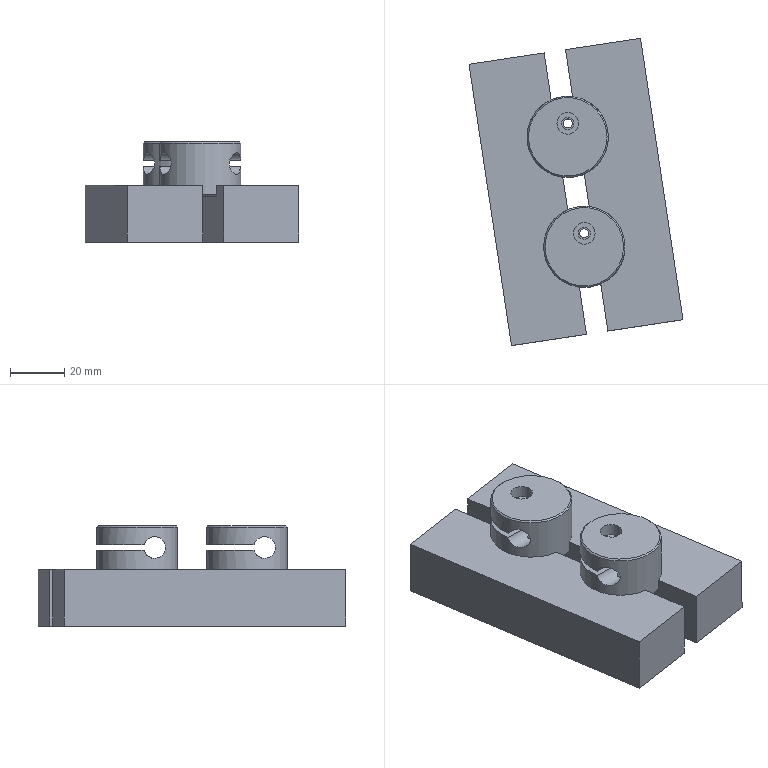Part | 4 solids | 54 faces | box 78.946 x 113.372 x 37 mm | volume 142342 mm3 | plane 26 | cylinder 24 | cone 4 | commonest cylinder face diameters 2.5 x10 30 x6 8 x4 3.3 x2 4.5 x2